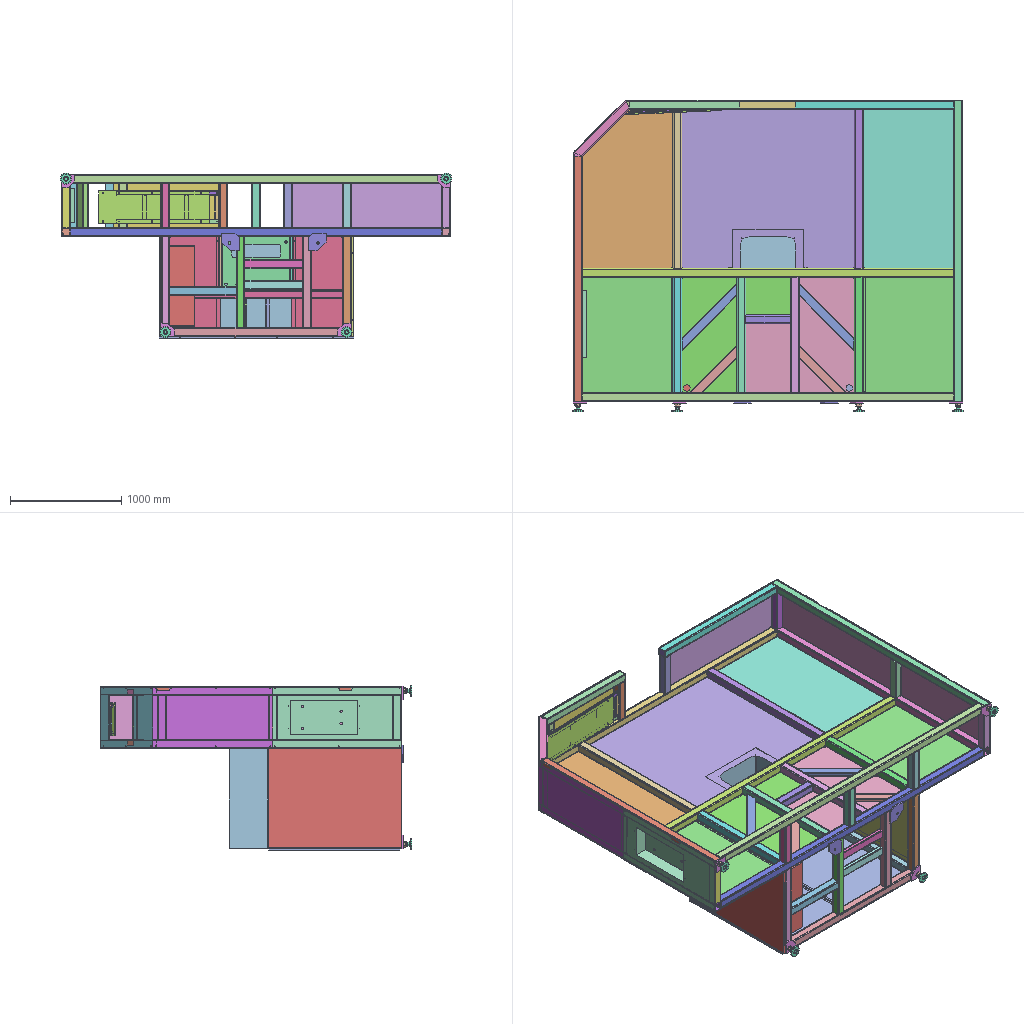Assembly | SolidWorks | 31 different items | 58 placed | box 3519 x 2801 x 1490 mm
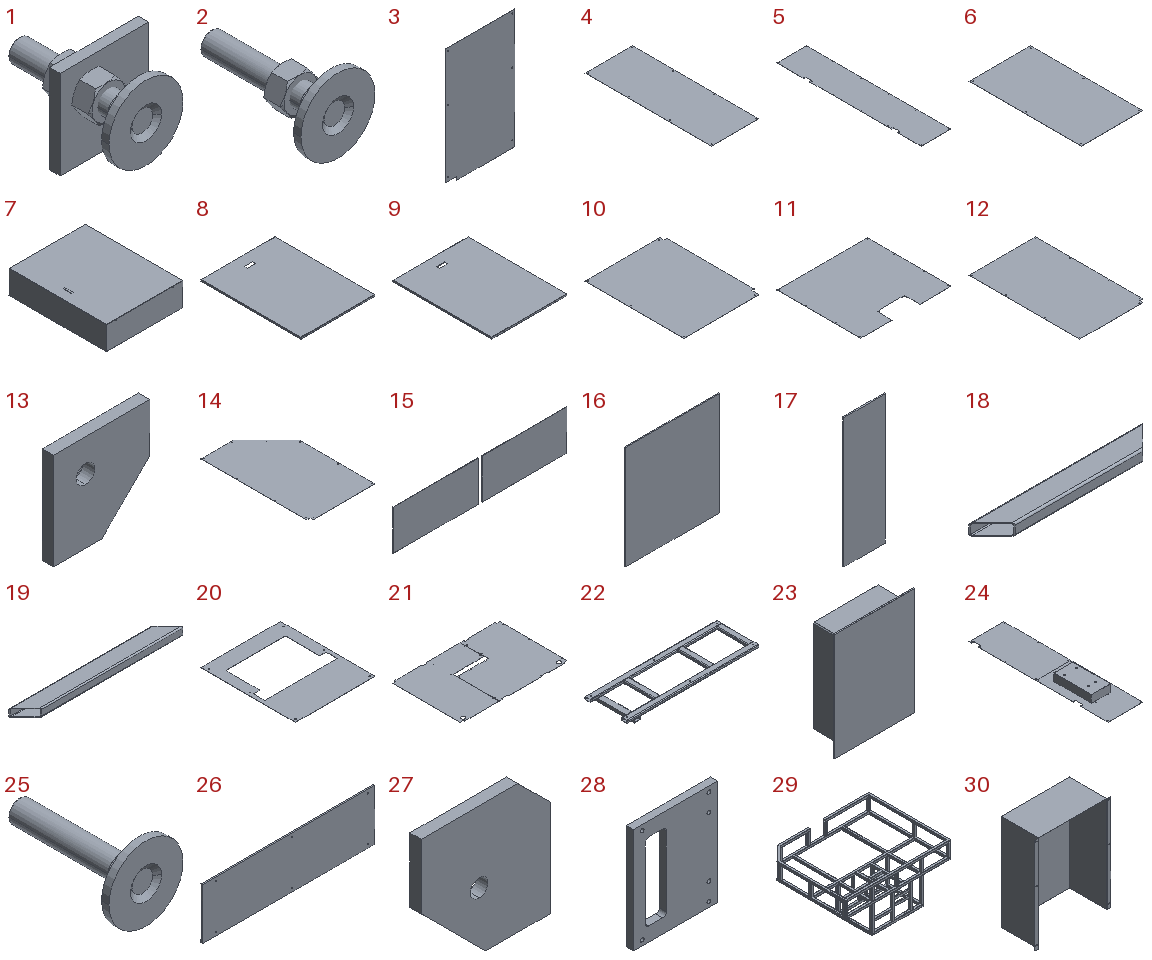Parts list (item | name | quantity | parent item | size | volume | features):
1 | (subassembly) | x4 | - | 130 x 171 x 130 mm | 461409 mm3 | -
2 | (subassembly) | x4 | in 1 | 100 x 171 x 100 mm | 248895 mm3 | -
3 | - | x2 | - | 535 x 1.2 x 915 mm | 584570 mm3 | features Fillet 4, ICE 4, FlatPattern 1, HoleWzd 1, SMBaseFlange 1, SheetMetal 1
4 | - | x1 | - | 560 x 1495 x 1.2 mm | 1004271 mm3 | features FlatPattern 1, HoleWzd 1, SMBaseFlange 1, SheetMetal 1
5 | - | x1 | - | 560 x 2710 x 1.2 mm | 1810338 mm3 | features Cut 1, Fillet 1, FlatPattern 1, HoleWzd 1, SMBaseFlange 1, SheetMetal 1
6 | - | x1 | - | 560 x 1020 x 1.2 mm | 685163 mm3 | features FlatPattern 1, HoleWzd 1, SMBaseFlange 1, SheetMetal 1
7 | - | x1 | - | 812 x 1034 x 255 mm | 2671023 mm3 | features ICE 9, EdgeFlange 2, LPattern 2, Emboss 1, FlatPattern 1, SMBaseFlange 1, SheetMetal 1
8 | - | x2 | - | 874 x 1178 x 20 mm | 1426991 mm3 | features ICE 6, EdgeFlange 4, CirPattern 2, FlatPattern 1, SMBaseFlange 1, SheetMetal 1
9 | - | x1 | - | 897 x 1178 x 20 mm | 1830546 mm3 | features EdgeFlange 2, ICE 2, FlatPattern 1, SMBaseFlange 1, SheetMetal 1
10 | - | x2 | - | 915 x 1162 x 1.2 mm | 1270668 mm3 | features Fillet 1, FlatPattern 1, HoleWzd 1, ICE 1, SMBaseFlange 1, SheetMetal 1
11 | - | x1 | - | 1628 x 1507 x 1.2 mm | 2778351 mm3 | features ICE 6, Fillet 3, HoleWzd 3, FlatPattern 1, SMBaseFlange 1, SheetMetal 1
12 | - | x1 | - | 933 x 1548 x 1.2 mm | 1730124 mm3 | features ICE 5, Fillet 2, FlatPattern 1, HoleWzd 1, SMBaseFlange 1, SheetMetal 1
13 | - | x4 | in 1 | 120 x 34 x 120 mm | 179889 mm3 | features ICE 2, Extrusion 1
14 | - | x1 | - | 933 x 1547 x 1.2 mm | 1597584 mm3 | features ICE 5, Fillet 3, HoleWzd 2, Cut 1, FlatPattern 1, SMBaseFlange 1, SheetMetal 1
15 | - | x1 | - | 1822 x 4 x 420 mm | 2993760 mm3 | features ICE 5, Extrusion 1
16 | - | x2 | - | 380 x 4 x 420 mm | 638400 mm3 | features Extrusion 1, ICE 1
17 | - | x2 | - | 135 x 4 x 420 mm | 226800 mm3 | features Extrusion 1, ICE 1
18 | - | x2 | - | 600 x 80 x 40 mm | 343628 mm3 | features 3DProfileFeature 1, ICE 1, WeldMemberFeat 1, WeldmentFeature 1
19 | - | x2 | - | 775 x 80 x 40 mm | 459272 mm3 | features 3DProfileFeature 1, ICE 1, WeldMemberFeat 1, WeldmentFeature 1
20 | - | x1 | - | 560 x 665 x 1.2 mm | 276730 mm3 | features Fillet 2, ICE 2, FlatPattern 1, HoleWzd 1, SMBaseFlange 1, SheetMetal 1
21 | - | x1 | - | 1632 x 1065 x 1.2 mm | 2027394 mm3 | features ICE 9, Fillet 5, FlatPattern 2, HoleWzd 1, SMBaseFlange 1, SheetMetal 1
22 | - | x1 | - | 920 x 295 x 40 mm | 708311 mm3 | features ICE 2, HoleWzd 1, WeldMemberFeat 1, WeldmentFeature 1
23 | - | x1 | - | 892 x 317 x 1197 mm | 3890024 mm3 | features ICE 2, Chamfer 1, Extrusion 1, Shell 1
24 | - | x1 | - | 560 x 2240 x 122 mm | 2071529 mm3 | features ICE 7, Fillet 4, HoleWzd 3, FlatPattern 2, SMBaseFlange 1, SheetMetal 1
25 | - | x4 | in 2 | 100 x 171 x 100 mm | 216271 mm3 | features ICE 3, Chamfer 1, RevCut 1, Revolution 1
26 | - | x1 | - | 995 x 10 x 295 mm | 2932412 mm3 | features Extrusion 1, HoleWzd 1
27 | - | x2 | - | 160 x 14 x 160 mm | 297078 mm3 | features ICE 2, BaseBody 1
28 | - | x1 | - | 480 x 40 x 600 mm | 9338608 mm3 | features Extrusion 1, Fillet 1, HoleWzd 1, ICE 1
29 | - | x1 | - | 3500 x 2710 x 1460 mm | 76195969 mm3 | features WeldCornerFeat 9, WeldMemberFeat 5, MoveCopyBody 4, ICE 2, 3DProfileFeature 1, EndCap 1, HoleWzd 1, WeldmentFeature 1
30 | - | x1 | - | 707.6 x 350 x 898 mm | 1775221 mm3 | features EdgeFlange 2, Fillet 1, FlatPattern 1, HoleWzd 1, ICE 1, SMBaseFlange 1, SheetMetal 1
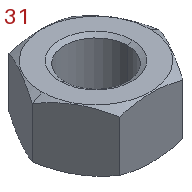31 | - | x8 | in 1, 2 | 53.116 x 46 x 25.6 mm | 32625 mm3 | features RevCut 2, Chamfer 1, Extrusion 1, LPattern 1
Mates (type | each side: item.copy, entity, surface, feature):
In the top assembly
Coincident | 26.1 face plane Boss-Extrude1 | assembly face | 3 times
DistanceDim | assembly face | assembly face | 11 times
Coincident | assembly face | assembly face | 15 times
Coincident | assembly face | 18.1 face plane Cut-Extrude1 | 2 times
DistanceDim | 18.1 face plane Cold-Formed Rect Hollow Section GB/T 6728-2002 80 X 40 X 3(1) | assembly face
Coincident | assembly face | 18.2 face plane Cut-Extrude1 | 2 times
Coincident | 18.1 face plane Cold-Formed Rect Hollow Section GB/T 6728-2002 80 X 40 X 3(1) | 18.2 face plane Cold-Formed Rect Hollow Section GB/T 6728-2002 80 X 40 X 3(1)
Coincident | assembly face | 5.1 face plane Base-Flange1 | 3 times
Coincident | assembly face | 12.1 face plane Base-Flange1
Coincident | 5.1 face plane Base-Flange1 | 12.1 face plane Base-Flange1 | 2 times
Coincident | assembly face | 14.1 face plane Base-Flange1 | 3 times
Coincident | assembly face | 11.1 face plane Base-Flange1 | 2 times
DistanceDim | 14.1 face plane Cut-Extrude4 | 11.1 face plane Cut-Extrude4
Coincident | assembly face | 10.1 face plane Base-Flange1 | 2 times
Coincident | 5.1 face plane Base-Flange1 | 10.1 face plane Base-Flange1
Coincident | assembly face | 10.2 face plane Base-Flange1 | 3 times
Coincident | assembly face | 3.1 face plane Base-Flange1 | 3 times
Coincident | 3.1 face plane Base-Flange1 | 30.1 face plane Edge-Flange2
Coincident | 11.1 face plane Base-Flange1 | 30.1 face plane Edge-Flange1
DistanceDim | assembly face | 10.1 face plane Base-Flange1
Coincident | assembly face | 7.1 face | 2 times
DistanceDim | 7.1 face | assembly face
Width | assembly face | assembly face | 30.1 face plane Edge-Flange1 | 30.1 face plane Edge-Flange1
Coincident | assembly face | 3.2 face plane Base-Flange1 | 2 times
Coincident | assembly face | 15.1 face plane Boss-Extrude1
DistanceDim | 15.1 face plane Boss-Extrude1 | assembly face | 2 times
Coincident | assembly face | 24.1 face plane Base-Flange1 | 3 times
PlanarAngleDim | 26.1 face plane Boss-Extrude1 | assembly face
DistanceDim | 26.1 face plane Boss-Extrude1 | assembly face
Coincident | assembly face | 29.1 face plane Square Tube 80 X 80 X 5.0(2) | 3 times
DistanceDim | 26.1 edge | 29.1 face plane Square Tube 80 X 80 X 5.0(2)
Coincident | 26.1 face plane Boss-Extrude1 | 22.1 face plane Rect Tube 40X20X2.5(1) | 2 times
Coincident | 29.1 face plane Square Tube 80 X 80 X 5.0(2) | 22.1 edge
Coincident | 29.1 face plane Square Tube 80 X 80 X 5.0(2) | 13.1 face plane Boss-Extrude1 | 3 times
Coincident | 29.1 face plane Square Tube 80 X 80 X 5.0(2) | 13.2 face plane Boss-Extrude1 | 3 times
Coincident | 29.1 face plane Square Tube 80 X 80 X 5.0(2) | 13.3 face plane Boss-Extrude1 | 3 times
Coincident | 29.1 face plane Square Tube 80 X 80 X 5.0(2) | 13.4 face plane Boss-Extrude1 | 3 times
Coincident | 27.1 face plane Input1 | 29.1 face plane Square Tube 80 X 80 X 5.0(2)
DistanceDim | 27.1 face plane Input1 | 29.1 face plane Square Tube 80 X 80 X 5.0(2) | 2 times
Coincident | 27.1 face plane Input1 | 27.2 face plane Input1
DistanceDim | 27.2 face plane Input1 | 29.1 face plane Square Tube 80 X 80 X 5.0(2) | 2 times
Coincident | 29.1 face plane Square Tube 80 X 80 X 5.0(2) | 21.1 face plane Base-Flange1
DistanceDim | 21.1 face plane Cut-Extrude4 | 29.1 face plane Square Tube 80 X 80 X 5.0(2)
DistanceDim | 21.1 face plane Base-Flange1 | 29.1 face plane Square Tube 80 X 80 X 5.0(2)
Coincident | 29.1 face plane Square Tube 80 X 80 X 5.0(2) | 20.1 face plane Base-Flange1 | 2 times
Coincident | 29.1 edge | 20.1 edge
Coincident | 29.1 face plane Square Tube 80 X 80 X 5.0(2) | 17.1 face plane Boss-Extrude1
Coincident | 29.1 face plane Square Tube 80 X 80 X 5.0(2) | 16.1 face plane Boss-Extrude1 | 2 times
Coincident | 17.1 face plane Boss-Extrude1 | 16.1 face plane Boss-Extrude1
Coincident | 29.1 face plane Square Tube 80 X 80 X 5.0(2) | 16.2 face plane Boss-Extrude1
DistanceDim | 16.2 face plane Boss-Extrude1 | 29.1 face plane Square Tube 80 X 80 X 5.0(2)
Coincident | 15.1 face plane Boss-Extrude1 | 16.2 face plane Boss-Extrude1
Coincident | 29.1 face plane Square Tube 80 X 80 X 5.0(2) | 17.2 face plane Boss-Extrude1
Coincident | 16.2 face plane Boss-Extrude1 | 17.2 face plane Boss-Extrude1
DistanceDim | 17.2 face plane Boss-Extrude1 | 16.2 face plane Boss-Extrude1
Coincident | 29.1 face plane Square Tube 80 X 80 X 5.0(2) | 5.2 face | 2 times
DistanceDim | 5.1 face plane Base-Flange1 | 5.2 face
Coincident | 29.1 face plane Square Tube 80 X 80 X 5.0(2) | 6.1 face plane Base-Flange1 | 2 times
Coincident | 29.1 face plane Square Tube 80 X 80 X 5.0(2) | 4.1 face plane Base-Flange1 | 2 times
Coincident | 5.1 face plane Base-Flange1 | 4.1 face plane Base-Flange1
Coincident | 29.1 face plane Rect Tube 80 X 40 X 4.0(1) | 28.1 face plane Boss-Extrude1 | 2 times
Coincident | 29.1 face plane Square Tube 80 X 80 X 5.0(2) | 28.1 face plane Boss-Extrude1
Coincident | 19.1 face plane Cut-Extrude1 | 29.1 face plane Square Tube 80 X 80 X 5.0(2)
Coincident | 10.1 face plane Base-Flange1 | 29.1 face plane Square Tube 80 X 80 X 5.0(2) | 2 times
DistanceDim | 19.2 face plane Cold-Formed Rect Hollow Section GB/T 6728-2002 80 X 40 X 3(1) | 29.1 face plane Square Tube 80 X 80 X 5.0(2)
Coincident | 5.1 face plane Base-Flange1 | 29.1 face plane Square Tube 80 X 80 X 5.0(2) | 3 times
Coincident | 12.1 face plane Base-Flange1 | 29.1 face plane Square Tube 80 X 80 X 5.0(2)
Coincident | 11.1 face plane Base-Flange1 | 29.1 face plane Square Tube 80 X 80 X 5.0(2)
Width | 11.1 face plane Cut-Extrude4 | 11.1 face plane Cut-Extrude4 | 29.1 face plane Square Tube 80 X 80 X 5.0(2) | 29.1 face plane Square Tube 80 X 80 X 5.0(2)
Coincident | 12.1 face plane Cut-Extrude2 | 11.1 face plane Cut-Extrude5
Coincident | 14.1 face plane Base-Flange1 | 29.1 face plane Square Tube 80 X 80 X 5.0(2)
Coincident | 14.1 face plane Cut-Extrude2 | 11.1 face plane Cut-Extrude5
Coincident | 24.1 face plane Base-Flange1 | 29.1 face plane Square Tube 80 X 80 X 5.0(2) | 3 times
Coincident | 10.2 face plane Base-Flange1 | 29.1 face plane Square Tube 80 X 80 X 5.0(2) | 2 times
Coincident | 10.2 face plane Base-Flange1 | 29.1 face plane Trim/Extend1
DistanceDim | 7.1 face | 29.1 face plane Square Tube 80 X 80 X 5.0(2)
Width | 7.1 face | 7.1 face | 29.1 face plane Square Tube 80 X 80 X 5.0(2) | 21.1 face plane Base-Flange1
DistanceDim | 16.1 face plane Boss-Extrude1 | 29.1 face plane Square Tube 80 X 80 X 5.0(2)
Slot | 3.2 face cylinder M6 Clearance Hole1 | 30.1 face cylinder Cut-Extrude1 | 2 times
Coincident | 3.2 face plane Base-Flange1 | 29.1 face plane Square Tube 80 X 80 X 5.0(2) | 2 times
Slot | 3.1 face cylinder M6 Clearance Hole1 | 30.1 face cylinder Cut-Extrude1 | 2 times
Coincident | 3.1 face plane Base-Flange1 | 29.1 face plane Square Tube 80 X 80 X 5.0(2)
Coincident | 10.1 face plane Base-Flange1 | 9.1 face plane Edge-Flange1
Coincident | 7.1 face | 29.1 face plane Square Tube 80 X 80 X 5.0(2)
Coincident | 29.1 face plane Square Tube 80 X 80 X 5.0(2) | 23.1 face plane Boss-Extrude2
Coincident | 14.1 face plane Base-Flange1 | 23.1 face plane Boss-Extrude1
Coincident | 29.1 face plane Square Tube 80 X 80 X 5.0(2) | 23.1 face plane Boss-Extrude1
Coincident | 20.1 edge | 6.1 face plane Base-Flange1
Coincident | 29.1 face plane Square Tube 80 X 80 X 5.0(2) | 8.1 face plane Edge-Flange2
Coincident | 9.1 face plane Edge-Flange1 | 8.1 face plane Edge-Flange1
Coincident | 9.1 face plane Base-Flange1 | 8.1 face plane Edge-Flange1
Coincident | 8.1 face plane Base-Flange1 | 8.2 face plane Base-Flange1
Coincident | 23.1 face plane Boss-Extrude1 | 8.2 face plane Edge-Flange1 | 2 times
Coincident | 8.1 face plane Edge-Flange1 | 8.2 face plane Edge-Flange1
In subassembly 1
Coincident | 13.5 face plane Boss-Extrude1 | 31.1 face plane BaseNut
Concentric | 13.5 face cylinder Cut-Extrude1 | 25.1 face cylinder Revolve1
Concentric | 25.1 face cylinder Revolve1 | 31.2 face cylinder BaseNut
Coincident | 13.5 face plane Boss-Extrude1 | 31.2 face plane BaseNut
In subassembly 2
Concentric | 25.2 face cylinder Revolve1 | 31.3 face cylinder BaseNut